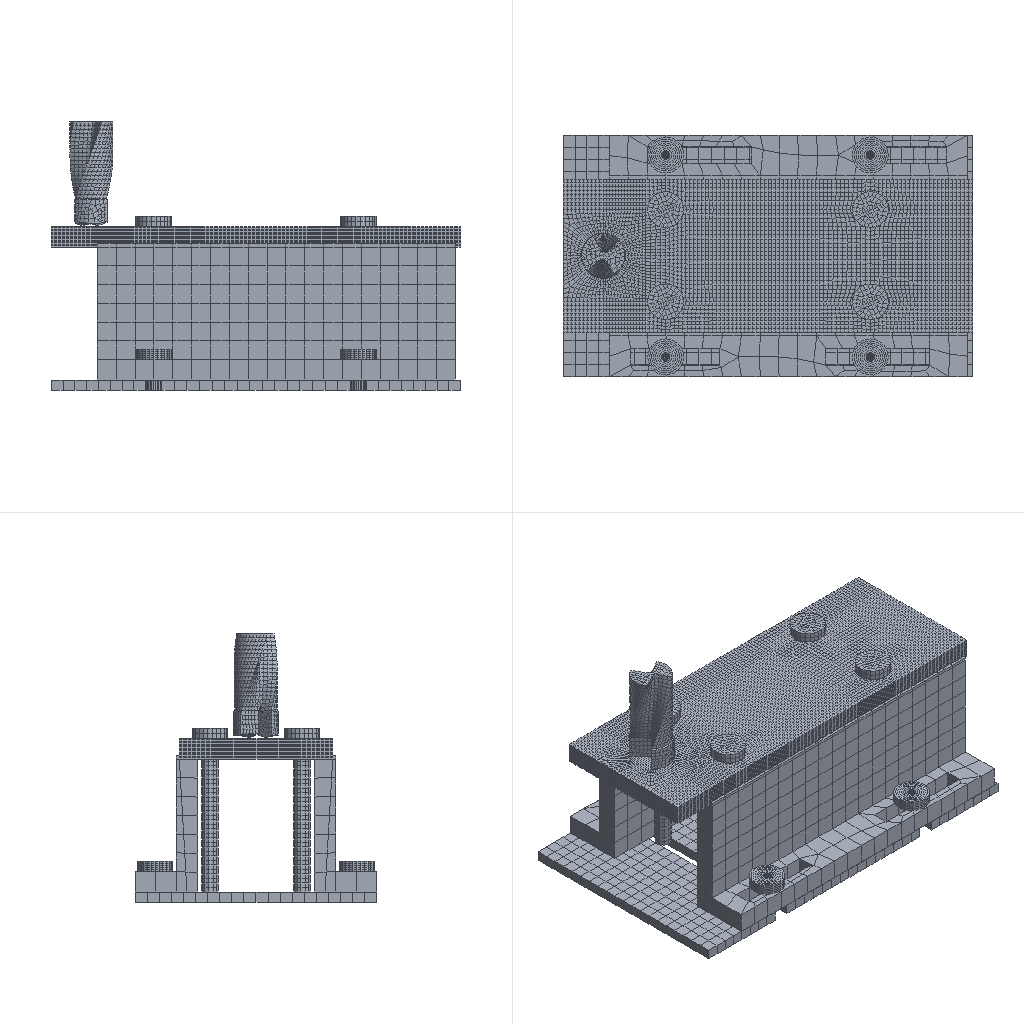Simulation study | abaqus
Set-up summary:
category,name,step,type,value,unit,region
solver,abaqus
solver,version,,,Abaqus/Standard 2024
units,not stated in the deck,,not stated
analysis,deck,,static,static
load_step,Step-1,Step-1,static,nlgeom=True
contact,interactions,,,general=0 pairs=22 ties=0
load_step,requested,,,1
mesh,nodes,,,96608
mesh,elements,,,84368
element_type,S3,,shell,42
element_type,S4R,,shell,1138
element_type,C3D8R,,solid,3884
element_type,C3D8RT,,solid,79304
load,load commands in deck,,count,4
bc,support commands in deck,,count,3
material,AL2219,,in results
material,AL2219-COPY,,in results
material,STEEL,,in results
check,setup vs results,,match,"per instance, exact: element labels, types and connectivity; labels of the nodes the elements use; coordinates of those nodes at SINGLE_PRECISION in 15 of 15 instance(s)"
Abaqus input file, long lists of numbers shortened, first 397 of 2407 lines:
*Heading
** Job name: yujing4 Model name: Model-1-Copy
** Generated by: Abaqus/CAE 2024
*Preprint, echo=NO, model=NO, history=NO, contact=NO
**
** PARTS
**
*Part, name=U44
*Node
      1,          76.,    14.767,  -16.307
      2,   97.892,    14.767,  -16.307
** (1159 more lines like these left out)
*Element, type=S4R
 1,   1,  57, 362,   4
 2,  57,  58, 363, 362
** (1136 more lines like these left out)
*Element, type=S3
873,   5,   6, 348
874, 344, 348,   6
** (40 more lines like these left out)
*Nset, nset=_PickedSet5, internal, generate
    1,  1161,     1
*Elset, elset=_PickedSet5, internal, generate
    1,  1180,     1
** Section: Section-4
*Shell Section, elset=_PickedSet5, material=steel
1., 5
*End Part
**
*Part, name=ban
*Node
      1,         150.,         -45.,           0.
      2,         150.,         -45.,          20.
** (71070 more lines like these left out)
*Element, type=C3D8RT
   1,  3164,  3165, 23216, 23000,   140,   139,  2928,  2927
   2,  3165,  3166, 23217, 23216,   139,   138,  2929,  2928
** (64018 more lines like these left out)
*Nset, nset=_PickedSet25, internal, generate
     1,  71072,      1
*Elset, elset=_PickedSet25, internal, generate
     1,  64020,      1
*Orientation, name=Ori-3
1., 0., 0., 0., 1., 0.
1, 0.
** Section: Section-2
*Solid Section, elset=_PickedSet25, orientation=Ori-3, material=AL2219
,
*End Part
**
*Part, name=diban1
*Node
      1,        -118.,          46.,           0.
      2,        -118.,         34.5,           0.
** (376 more lines like these left out)
*Element, type=C3D8R
  1,  19,  20,  29,  28,   1,   2,  11,  10
  2,  20,  21,  30,  29,   2,   3,  12,  11
** (158 more lines like these left out)
*Node
    379,           0.,           0.,          10.
*Nset, nset=diban1-RefPt_, internal
379,
*Nset, nset=_PickedSet2, internal, generate
   1,  378,    1
*Elset, elset=_PickedSet2, internal, generate
   1,  160,    1
** Section: steel
*Solid Section, elset=_PickedSet2, material=steel
,
*End Part
**
*Part, name=diban2
*Node
      1,        -118.,           0.,         -92.
      2,        -118.,           0.,  -79.733
** (670 more lines like these left out)
*Element, type=C3D8R
  1,  33,  34,  50,  49,   1,   2,  18,  17
  2,  34,  35,  51,  50,   2,   3,  19,  18
** (298 more lines like these left out)
*Node
    673,           0.,          10.,           0.
*Nset, nset=diban2-RefPt_, internal
673,
*Nset, nset=_PickedSet2, internal, generate
   1,  672,    1
*Elset, elset=_PickedSet2, internal, generate
   1,  300,    1
** Section: steel
*Solid Section, elset=_PickedSet2, material=steel
,
*End Part
**
*Part, name=dizuo
*Node
      1,   10.508,  -254.413,           0.
      2,   10.508,   95.587,           0.
** (650 more lines like these left out)
*Element, type=C3D8RT
  1,  11, 151, 545, 299,   1,  37, 281,  74
  2, 151, 152, 546, 545,  37,  38, 282, 281
** (336 more lines like these left out)
*Nset, nset=_PickedSet9, internal, generate
   1,  652,    1
*Elset, elset=_PickedSet9, internal, generate
   1,  338,    1
*Orientation, name=Ori-1
1., 0., 0., 0., 1., 0.
1, 0.
** Section: Section-3
*Solid Section, elset=_PickedSet9, orientation=Ori-1, material=AL2219-Copy
,
*End Part
**
*Part, name=luoshuan
*Node
      1,           0.,          -8.,          85.
      2,           0.,           0.,          85.
** (1159 more lines like these left out)
*Element, type=C3D8R
 1, 312, 313, 883, 874,  25,  26, 295, 294
 2, 313,  28, 296, 883,  26,   1,  27, 295
** (814 more lines like these left out)
*Nset, nset=_PickedSet2, internal, generate
    1,  1161,     1
*Elset, elset=_PickedSet2, internal, generate
   1,  816,    1
** Section: steel
*Solid Section, elset=_PickedSet2, material=steel
,
*End Part
**
*Part, name=luoshuan2
*Node
      1,           0.,          40.,  -4.142
      2,           0.,          40.,          -8.
** (4247 more lines like these left out)
*Element, type=C3D8RT
  1,  370,  397,   27,   28, 1840, 1867,  603,  604
  2,  374,   68,   69,  373, 1844,  452,  451, 1843
** (3650 more lines like these left out)
*Nset, nset=_PickedSet2, internal, generate
    1,  4249,     1
*Elset, elset=_PickedSet2, internal, generate
    1,  3652,     1
** Section: steel
*Solid Section, elset=_PickedSet2, material=steel
,
*End Part
**
**
** ASSEMBLY
**
*Assembly, name=Assembly
**
*Instance, name=diban2, part=diban2
-0.5575, 2.091,        -140.
-0.5575, 2.091,        -140., 0.01987, 2.668, -140.577,         240.
*End Instance
**
*Instance, name=luoshuan2, part=luoshuan2
99.443, -96.588,        -110.
99.443, -96.588,        -110., 98.443, -96.588,        -110., 90.
*End Instance
**
*Instance, name=luoshuan2_1, part=luoshuan2
99.443, 100.769,        -110.
99.443, 100.769,        -110., 98.443, 100.769,        -110., 90.
*End Instance
**
*Instance, name=diban1, part=diban1
153.443, 2.091,        -150.
153.443, 2.091,        -150., 153.443, 2.091, -149., 90.
*End Instance
**
*Instance, name=luoshuan2_2, part=luoshuan2
-100.557, 100.769,        -110.
-100.557, 100.769,        -110., -101.557, 100.769,        -110., 90.
*End Instance
**
*Instance, name=luoshuan2_3, part=luoshuan2
-100.557, -96.588,        -110.
-100.557, -96.588,        -110., -101.557, -96.588,        -110., 90.
*End Instance
**
*Instance, name=diban1_4, part=diban1
-154.557, 2.091,        -150.
-154.557, 2.091,        -150., -154.557, 2.091, -151., 90.
*End Instance
**
*Instance, name=dizuo, part=dizuo
-59.971, -86.418,        -140.
-59.971, -86.418,        -140., -59.971, -86.418, -139., 90.
*End Instance
**
*Instance, name=dizuo_5, part=dizuo
98.856, 90.599,        -140.
98.856, 90.599,        -140., 98.856, 90.599, -141., 90.
*End Instance
**
*Instance, name=luoshuan, part=luoshuan
99.443, 47.091,          20.
99.443, 47.091,          20., 99.247, 48.071,          20.,         180.
*End Instance
**
*Instance, name=luoshuan_6, part=luoshuan
99.443, -42.909,          20.
99.443, -42.909,          20., 99.247, -41.929,          20.,         180.
*End Instance
**
*Instance, name=luoshuan_7, part=luoshuan
-100.557, -42.909,          20.
-100.557, -42.909,          20., -100.753, -41.929,          20.,         180.
*End Instance
**
*Instance, name=luoshuan_8, part=luoshuan
-100.557, 47.091,          20.
-100.557, 47.091,          20., -100.753, 48.071,          20.,         180.
*End Instance
**
*Instance, name=ban, part=ban
-0.5575, 2.091,         -10.
*End Instance
**
*Instance, name=temp-U44钻头2025-2-new-1, part=U44
-161.557, 2.091, 112.448
-161.557, 2.091, 112.448, -161.557, 3.091, 112.448, 90.
*End Instance
**
*Nset, nset=Set-2, instance=ban
   107,   108,   109,   110,   119,   120,   122,   123,   129,   130,  2203,  2204,  2205,  2206,  2207,  2208
  2209,  2210,  2211,  2212,  2213,  2214,  2215,  2216,  2217,  2218,  2219,  2220,  2221,  2222,  2223,  2224
** (389 more lines like these left out)
*Nset, nset=_PickedSet283, internal, instance=luoshuan2
    1,    2,    7,    8,   15,   16,   21,   22,   26,   80,   81,   82,   83,   84,   85,   92
   93,   94,   95,   96,   97,  110,  170,  171,  172,  173,  174,  175,  176,  177,  178,  179
** (8 more lines like these left out)
*Nset, nset=_PickedSet283, internal, instance=luoshuan2_1
    1,    2,    7,    8,   15,   16,   21,   22,   26,   80,   81,   82,   83,   84,   85,   92
   93,   94,   95,   96,   97,  110,  170,  171,  172,  173,  174,  175,  176,  177,  178,  179
** (8 more lines like these left out)
*Nset, nset=_PickedSet283, internal, instance=luoshuan2_3
    1,    2,    7,    8,   15,   16,   21,   22,   26,   80,   81,   82,   83,   84,   85,   92
   93,   94,   95,   96,   97,  110,  170,  171,  172,  173,  174,  175,  176,  177,  178,  179
** (8 more lines like these left out)
*Nset, nset=_PickedSet283, internal, instance=luoshuan2_2
    1,    2,    7,    8,   15,   16,   21,   22,   26,   80,   81,   82,   83,   84,   85,   92
   93,   94,   95,   96,   97,  110,  170,  171,  172,  173,  174,  175,  176,  177,  178,  179
** (8 more lines like these left out)
*Elset, elset=_PickedSet283, internal, instance=luoshuan2
    5,   32,   74,  101,  143,  170,  212,  239,  281,  308,  350,  377,  419,  446,  488,  515
  557,  584,  626,  653,  695,  722,  764,  791,  833,  860,  902,  929,  971,  998, 1040, 1067
** (7 more lines like these left out)
*Elset, elset=_PickedSet283, internal, instance=luoshuan2_1
    5,   32,   74,  101,  143,  170,  212,  239,  281,  308,  350,  377,  419,  446,  488,  515
  557,  584,  626,  653,  695,  722,  764,  791,  833,  860,  902,  929,  971,  998, 1040, 1067
** (7 more lines like these left out)
*Elset, elset=_PickedSet283, internal, instance=luoshuan2_3
    5,   32,   74,  101,  143,  170,  212,  239,  281,  308,  350,  377,  419,  446,  488,  515
  557,  584,  626,  653,  695,  722,  764,  791,  833,  860,  902,  929,  971,  998, 1040, 1067
** (7 more lines like these left out)
*Elset, elset=_PickedSet283, internal, instance=luoshuan2_2
    5,   32,   74,  101,  143,  170,  212,  239,  281,  308,  350,  377,  419,  446,  488,  515
  557,  584,  626,  653,  695,  722,  764,  791,  833,  860,  902,  929,  971,  998, 1040, 1067
** (7 more lines like these left out)
*Nset, nset=_PickedSet284, internal, instance=luoshuan
   4,   5,   6,   8,  10,  78,  79,  80,  81,  82, 103, 104, 105, 106, 126, 127
 128, 223, 224, 376, 377, 444, 445, 496, 497, 730, 731
*Nset, nset=_PickedSet284, internal, instance=luoshuan_6
   4,   5,   6,   8,  10,  78,  79,  80,  81,  82, 103, 104, 105, 106, 126, 127
 128, 223, 224, 376, 377, 444, 445, 496, 497, 730, 731
*Nset, nset=_PickedSet284, internal, instance=luoshuan_7
   4,   5,   6,   8,  10,  78,  79,  80,  81,  82, 103, 104, 105, 106, 126, 127
 128, 223, 224, 376, 377, 444, 445, 496, 497, 730, 731
*Nset, nset=_PickedSet284, internal, instance=luoshuan_8
   4,   5,   6,   8,  10,  78,  79,  80,  81,  82, 103, 104, 105, 106, 126, 127
 128, 223, 224, 376, 377, 444, 445, 496, 497, 730, 731
*Elset, elset=_PickedSet284, internal, instance=luoshuan
  49,  58,  59,  68,  85, 134, 135, 136, 161, 170, 219, 220, 221, 246, 255, 545
 553, 554, 580, 581
*Elset, elset=_PickedSet284, internal, instance=luoshuan_6
  49,  58,  59,  68,  85, 134, 135, 136, 161, 170, 219, 220, 221, 246, 255, 545
 553, 554, 580, 581
*Elset, elset=_PickedSet284, internal, instance=luoshuan_7
  49,  58,  59,  68,  85, 134, 135, 136, 161, 170, 219, 220, 221, 246, 255, 545
 553, 554, 580, 581
*Elset, elset=_PickedSet284, internal, instance=luoshuan_8
  49,  58,  59,  68,  85, 134, 135, 136, 161, 170, 219, 220, 221, 246, 255, 545
 553, 554, 580, 581
*Nset, nset=_PickedSet291, internal, instance=diban2
 673,
*Nset, nset=_PickedSet291, internal, instance=diban1
 379,
*Nset, nset=_PickedSet291, internal, instance=diban1_4
 379,
*Nset, nset=_PickedSet292, internal, instance=diban1_4
 379,
*Nset, nset=_PickedSet293, internal, instance=diban1_4, generate
   1,  378,    1
*Elset, elset=_PickedSet293, internal, instance=diban1_4, generate
   1,  160,    1
*Nset, nset=_PickedSet294, internal, instance=diban2
 673,
*Nset, nset=_PickedSet295, internal, instance=diban2, generate
   1,  672,    1
*Elset, elset=_PickedSet295, internal, instance=diban2, generate
   1,  300,    1
*Nset, nset=_PickedSet296, internal, instance=diban1
 379,
*Nset, nset=_PickedSet297, internal, instance=diban1, generate
   1,  378,    1
*Elset, elset=_PickedSet297, internal, instance=diban1, generate
   1,  160,    1
*Elset, elset=_CP-1-diban2_S3, internal, instance=diban2, generate
   1,  300,    1
*Surface, type=ELEMENT, name=CP-1-diban2
_CP-1-diban2_S3, S3
*Elset, elset=_CP-1-dizuo_S1, internal, instance=dizuo, generate
 286,  338,    1
*Elset, elset=_CP-1-dizuo_S2, internal, instance=dizuo, generate
  1,  38,   1
*Surface, type=ELEMENT, name=CP-1-dizuo
_CP-1-dizuo_S1, S1
_CP-1-dizuo_S2, S2
*Elset, elset=_CP-2-diban2_S3, internal, instance=diban2, generate
   1,  300,    1
*Surface, type=ELEMENT, name=CP-2-diban2
_CP-2-diban2_S3, S3
*Elset, elset=_CP-2-dizuo_S1, internal, instance=dizuo, generate
 286,  338,    1
*Elset, elset=_CP-2-dizuo_S2, internal, instance=dizuo, generate
  1,  38,   1
*Surface, type=ELEMENT, name=CP-2-dizuo
_CP-2-dizuo_S1, S1
_CP-2-dizuo_S2, S2
*Elset, elset=_CP-2-dizuo_5_S1, internal, instance=dizuo_5, generate
 286,  338,    1
*Elset, elset=_CP-2-dizuo_5_S2, internal, instance=dizuo_5, generate
  1,  38,   1
*Surface, type=ELEMENT, name=CP-2-dizuo_5
_CP-2-dizuo_5_S1, S1
_CP-2-dizuo_5_S2, S2
*Elset, elset=_CP-3-diban2_S3, internal, instance=diban2, generate
   1,  300,    1
*Surface, type=ELEMENT, name=CP-3-diban2
_CP-3-diban2_S3, S3
*Elset, elset=_CP-3-dizuo_S2, internal, instance=dizuo, generate
 286,  338,    1
*Surface, type=ELEMENT, name=CP-3-dizuo
_CP-3-dizuo_S2, S2
*Elset, elset=_CP-3-dizuo_5_S1, internal, instance=dizuo_5, generate
 286,  338,    1
*Elset, elset=_CP-3-dizuo_5_S2, internal, instance=dizuo_5, generate
  1,  38,   1
*Surface, type=ELEMENT, name=CP-3-dizuo_5
_CP-3-dizuo_5_S1, S1
_CP-3-dizuo_5_S2, S2
*Elset, elset=_CP-3-luoshuan2_S3, internal, instance=luoshuan2
   19,   21,   49,   51,   88,   90,  118,  120,  157,  159,  187,  189,  226,  228,  256,  258
  295,  297,  325,  327,  364,  366,  394,  396,  433,  435,  463,  465,  502,  504,  532,  534
** (5 more lines like these left out)
*Elset, elset=_CP-3-luoshuan2_S5, internal, instance=luoshuan2, generate
   22,  1885,    69
*Surface, type=ELEMENT, name=CP-3-luoshuan2
_CP-3-luoshuan2_S3, S3
_CP-3-luoshuan2_S5, S5
*Elset, elset=_CP-4-diban2_S3, internal, instance=diban2, generate
   1,  300,    1
*Surface, type=ELEMENT, name=CP-4-diban2
_CP-4-diban2_S3, S3
*Elset, elset=_CP-4-dizuo_S4, internal, instance=dizuo
 292, 306
*Elset, elset=_CP-4-dizuo_S6, internal, instance=dizuo
 305, 307, 315, 316
*Surface, type=ELEMENT, name=CP-4-dizuo
_CP-4-dizuo_S4, S4
_CP-4-dizuo_S6, S6
*Elset, elset=_CP-4-dizuo_5_S1, internal, instance=dizuo_5, generate
 286,  338,    1
*Elset, elset=_CP-4-dizuo_5_S2, internal, instance=dizuo_5, generate
  1,  38,   1
*Surface, type=ELEMENT, name=CP-4-dizuo_5
_CP-4-dizuo_5_S1, S1
_CP-4-dizuo_5_S2, S2
*Elset, elset=_CP-4-luoshuan2_S5, internal, instance=luoshuan2
    1,    7,    8,    9,   10,   11,   12,   13,   14,   15,   16,   17,   18,   59,   70,   76
   77,   78,   79,   80,   81,   82,   83,   84,   85,   86,   87,  128,  139,  145,  146,  147
** (23 more lines like these left out)
*Elset, elset=_CP-4-luoshuan2_S3, internal, instance=luoshuan2, generate
    5,  1868,    69
*Surface, type=ELEMENT, name=CP-4-luoshuan2
_CP-4-luoshuan2_S5, S5
_CP-4-luoshuan2_S3, S3
*Elset, elset=_CP-5-diban2_S3, internal, instance=diban2, generate
   1,  300,    1
*Surface, type=ELEMENT, name=CP-5-diban2
Last 646 lines:
   366,   372,   378,   384,   390,   396,   402,   408,   414,   420,   426,   432,   438,   444,   450,   456
   462,   468,   474,   480,   486,   492,   498,   504,   510,   516,   522,   528,   534,   540,   546,   552
** (18 more lines like these left out)
*Elset, elset=_CP-40-ban_S2, internal, instance=ban
 22126, 22127, 22128, 22129, 22130, 22131, 22132, 22133, 22134, 22135, 22136, 22137, 22138, 22139, 22140, 22141
 22222, 22223, 22224, 22225, 22226, 22227, 22228, 22229, 22230, 22231, 22232, 22233, 22234, 22235, 39413, 39414
** (11 more lines like these left out)
*Elset, elset=_CP-40-ban_S6, internal, instance=ban, generate
 35866,  37418,      8
*Surface, type=ELEMENT, name=CP-40-ban
_CP-40-ban_S5, S5
_CP-40-ban_S3, S3
_CP-40-ban_S4, S4
_CP-40-ban_S2, S2
_CP-40-ban_S6, S6
*Elset, elset=_CP-40-dizuo_S2, internal, instance=dizuo, generate
 286,  338,    1
*Surface, type=ELEMENT, name=CP-40-dizuo
_CP-40-dizuo_S2, S2
*Elset, elset=_CP-40-dizuo_5_S4, internal, instance=dizuo_5
 292, 306
*Elset, elset=_CP-40-dizuo_5_S6, internal, instance=dizuo_5
 305, 307, 315, 316
*Surface, type=ELEMENT, name=CP-40-dizuo_5
_CP-40-dizuo_5_S4, S4
_CP-40-dizuo_5_S6, S6
*Elset, elset=_CP-41-ban_S6, internal, instance=ban
  5551,  5566,  5581,  5596,  5611,  5626,  5641,  5656,  5671,  5686,  5701,  5716,  5731,  5746,  5761,  5776
  5791,  5806,  5821,  5836,  5851,  5866,  5881,  5896,  5911,  5926,  5941,  5956,  5971,  5986,  6001,  6016
** (66 more lines like these left out)
*Elset, elset=_CP-41-ban_S5, internal, instance=ban
  9410,  9411,  9412,  9413,  9414,  9415,  9416,  9417,  9418,  9419,  9420,  9575,  9576,  9577,  9578,  9579
  9580,  9581,  9582,  9583,  9584,  9585,  9740,  9741,  9742,  9743,  9744,  9745,  9746,  9747,  9748,  9749
** (7 more lines like these left out)
*Elset, elset=_CP-41-ban_S4, internal, instance=ban
     8,    16,    24,    32,    40,    48,    56,    64,    72,    80,    88,    96,   104,   112,   120,   128
   136,   144,   152,   160,   168,   176,   830,   838,   846,   854,   862,   870,   878,   886,   894,   902
** (104 more lines like these left out)
*Elset, elset=_CP-41-ban_S3, internal, instance=ban
   345,   353,  1449,  1450,  1465,  1466,  1467,  1468,  1469,  1470,  1513,  1514,  1515,  1516,  1517,  1518
  2881,  2882,  2883,  2902,  2903,  2904,  2923,  2924,  2925,  2944,  2945,  2946,  2965,  2966,  2967,  2986
** (55 more lines like these left out)
*Elset, elset=_CP-41-ban_S2, internal, instance=ban
  3549, 12586, 12587, 12602, 12603, 12604, 12605, 12606, 12607, 12608, 12609, 12610, 12611, 18916, 18917, 18918
 18919, 18920, 18921, 18922, 18923, 18924, 18925, 18996, 18997, 20791, 20792, 20793, 20794, 20795, 20796, 20797
** (27 more lines like these left out)
*Surface, type=ELEMENT, name=CP-41-ban
_CP-41-ban_S6, S6
_CP-41-ban_S5, S5
_CP-41-ban_S4, S4
_CP-41-ban_S2, S2
_CP-41-ban_S3, S3
*Elset, elset=_CP-41-dizuo_S1, internal, instance=dizuo, generate
 286,  338,    1
*Elset, elset=_CP-41-dizuo_S2, internal, instance=dizuo, generate
  1,  38,   1
*Surface, type=ELEMENT, name=CP-41-dizuo
_CP-41-dizuo_S1, S1
_CP-41-dizuo_S2, S2
*Elset, elset=_CP-41-dizuo_5_S2, internal, instance=dizuo_5, generate
 286,  338,    1
*Surface, type=ELEMENT, name=CP-41-dizuo_5
_CP-41-dizuo_5_S2, S2
*Elset, elset=_CP-42-ban_S4, internal, instance=ban
 11735, 11740, 11745, 11750, 11755, 11760, 11765, 11770, 11775, 11780, 11785, 11790, 11795, 11800, 11805, 11810
 11815, 11820, 11825, 11830, 11835, 11840, 11845, 11850, 11855, 11860, 11865, 11870, 11875, 11880, 11885, 11890
** (21 more lines like these left out)
*Elset, elset=_CP-42-ban_S3, internal, instance=ban
 12171, 12172, 12173, 12174, 12175, 12176, 12177, 12206, 12207, 12208, 12209, 12210, 12211, 12212, 12241, 12242
 12243, 12244, 12245, 12246, 12247, 12276, 12277, 12278, 12279, 12280, 12281, 12282, 12311, 12312, 12313, 12314
** (16 more lines like these left out)
*Elset, elset=_CP-42-ban_S5, internal, instance=ban
 12856, 12857, 12858, 12859, 12860, 12861, 12862, 12863, 12864, 12865, 12866, 12867, 12868, 12869, 12870, 12961
 12962, 12963, 12964, 12965, 12966, 12967, 12968, 12969, 12970, 12971, 12972, 12973, 12974, 12975, 13066, 13067
** (36 more lines like these left out)
*Elset, elset=_CP-42-ban_S2, internal, instance=ban
 19012, 19013, 19014, 19015, 19016, 19017, 19018, 19019, 19020, 19021, 19022, 19023, 19024, 19025, 46141, 46142
 46143, 46144, 46145, 46146, 46147, 46148, 46149, 46150, 46151, 46152, 46153, 46154, 46155, 46156, 46157, 46158
** (21 more lines like these left out)
*Surface, type=ELEMENT, name=CP-42-ban
_CP-42-ban_S4, S4
_CP-42-ban_S3, S3
_CP-42-ban_S2, S2
_CP-42-ban_S5, S5
*Elset, elset=_CP-42-dizuo_S1, internal, instance=dizuo, generate
 248,  266,    1
*Surface, type=ELEMENT, name=CP-42-dizuo
_CP-42-dizuo_S1, S1
*Elset, elset=_CP-42-dizuo_5_S1, internal, instance=dizuo_5, generate
 286,  338,    1
*Elset, elset=_CP-42-dizuo_5_S2, internal, instance=dizuo_5, generate
  1,  38,   1
*Surface, type=ELEMENT, name=CP-42-dizuo_5
_CP-42-dizuo_5_S1, S1
_CP-42-dizuo_5_S2, S2
*Elset, elset=_CP-43-ban_S3, internal, instance=ban
   177,   178,   179,   180,   181,   182,   183,   184,   185,   186,   187,   254,   255,   256,   257,   258
   259,   260,   261,   262,   263,   264,   361,   362,   363,   364,   365,   366,   403,   404,   405,   406
** (88 more lines like these left out)
*Elset, elset=_CP-43-ban_S4, internal, instance=ban
   337,   344,  3119,  3127,  3135,  3143,  3151,  3159,  3167,  3175,  3183,  3191,  3199,  3207,  3215,  3223
  3231,  3239,  3247,  3255,  3263,  3271,  3279,  3287,  3295,  3303,  3311,  3319,  3327,  3335,  3343,  3351
** (116 more lines like these left out)
*Elset, elset=_CP-43-ban_S2, internal, instance=ban
  1351,  1352,  1365,  1366,  1367,  1368,  1369,  1370,  1371,  1372,  1373,  1374,  1375,  1376,  3496,  3497
  3498,  3520,  5371,  5372,  5373,  5374,  5375,  5376,  5377,  5378,  5427,  5434,  5435,  5436, 19082, 19083
** (20 more lines like these left out)
*Elset, elset=_CP-43-ban_S6, internal, instance=ban
  7111,  7126,  7141,  7156,  7171,  7186,  7201,  7216,  7231,  7246,  7261,  7276,  7291,  7306,  7321,  7336
  7351,  7366,  7381,  7396,  7411,  7426,  7441,  7456,  7471,  7486,  7501,  7516,  7531,  7546,  7561,  7576
** (30 more lines like these left out)
*Elset, elset=_CP-43-ban_S1, internal, instance=ban, generate
 37322,  37425,      1
*Surface, type=ELEMENT, name=CP-43-ban
_CP-43-ban_S3, S3
_CP-43-ban_S4, S4
_CP-43-ban_S2, S2
_CP-43-ban_S6, S6
_CP-43-ban_S1, S1
*Elset, elset=_CP-43-dizuo_S6, internal, instance=dizuo, generate
 267,  285,    1
*Surface, type=ELEMENT, name=CP-43-dizuo
_CP-43-dizuo_S6, S6
*Elset, elset=_CP-43-dizuo_5_S1, internal, instance=dizuo_5, generate
 248,  266,    1
*Surface, type=ELEMENT, name=CP-43-dizuo_5
_CP-43-dizuo_5_S1, S1
*Elset, elset=_CP-44-ban_S3, internal, instance=ban
   177,   178,   179,   180,   181,   182,   183,   184,   185,   186,   187,   254,   255,   256,   257,   258
   259,   260,   261,   262,   263,   264,   361,   362,   363,   364,   365,   366,   403,   404,   405,   406
** (88 more lines like these left out)
*Elset, elset=_CP-44-ban_S4, internal, instance=ban
   337,   344,  3119,  3127,  3135,  3143,  3151,  3159,  3167,  3175,  3183,  3191,  3199,  3207,  3215,  3223
  3231,  3239,  3247,  3255,  3263,  3271,  3279,  3287,  3295,  3303,  3311,  3319,  3327,  3335,  3343,  3351
** (116 more lines like these left out)
*Elset, elset=_CP-44-ban_S2, internal, instance=ban
  1351,  1352,  1365,  1366,  1367,  1368,  1369,  1370,  1371,  1372,  1373,  1374,  1375,  1376,  3496,  3497
  3498,  3520,  5371,  5372,  5373,  5374,  5375,  5376,  5377,  5378,  5427,  5434,  5435,  5436, 19082, 19083
** (20 more lines like these left out)
*Elset, elset=_CP-44-ban_S6, internal, instance=ban
  7111,  7126,  7141,  7156,  7171,  7186,  7201,  7216,  7231,  7246,  7261,  7276,  7291,  7306,  7321,  7336
  7351,  7366,  7381,  7396,  7411,  7426,  7441,  7456,  7471,  7486,  7501,  7516,  7531,  7546,  7561,  7576
** (30 more lines like these left out)
*Elset, elset=_CP-44-ban_S1, internal, instance=ban, generate
 37322,  37425,      1
*Surface, type=ELEMENT, name=CP-44-ban
_CP-44-ban_S3, S3
_CP-44-ban_S4, S4
_CP-44-ban_S2, S2
_CP-44-ban_S6, S6
_CP-44-ban_S1, S1
*Elset, elset=_CP-44-dizuo_5_S6, internal, instance=dizuo_5, generate
 267,  285,    1
*Surface, type=ELEMENT, name=CP-44-dizuo_5
_CP-44-dizuo_5_S6, S6
*Elset, elset=_CP-45-ban_S3, internal, instance=ban
   177,   178,   179,   180,   181,   182,   183,   184,   185,   186,   187,   254,   255,   256,   257,   258
   259,   260,   261,   262,   263,   264,   361,   362,   363,   364,   365,   366,   403,   404,   405,   406
** (88 more lines like these left out)
*Elset, elset=_CP-45-ban_S4, internal, instance=ban
   337,   344,  3119,  3127,  3135,  3143,  3151,  3159,  3167,  3175,  3183,  3191,  3199,  3207,  3215,  3223
  3231,  3239,  3247,  3255,  3263,  3271,  3279,  3287,  3295,  3303,  3311,  3319,  3327,  3335,  3343,  3351
** (116 more lines like these left out)
*Elset, elset=_CP-45-ban_S2, internal, instance=ban
  1351,  1352,  1365,  1366,  1367,  1368,  1369,  1370,  1371,  1372,  1373,  1374,  1375,  1376,  3496,  3497
  3498,  3520,  5371,  5372,  5373,  5374,  5375,  5376,  5377,  5378,  5427,  5434,  5435,  5436, 19082, 19083
** (20 more lines like these left out)
*Elset, elset=_CP-45-ban_S6, internal, instance=ban
  7111,  7126,  7141,  7156,  7171,  7186,  7201,  7216,  7231,  7246,  7261,  7276,  7291,  7306,  7321,  7336
  7351,  7366,  7381,  7396,  7411,  7426,  7441,  7456,  7471,  7486,  7501,  7516,  7531,  7546,  7561,  7576
** (30 more lines like these left out)
*Elset, elset=_CP-45-ban_S1, internal, instance=ban, generate
 37322,  37425,      1
*Surface, type=ELEMENT, name=CP-45-ban
_CP-45-ban_S3, S3
_CP-45-ban_S4, S4
_CP-45-ban_S2, S2
_CP-45-ban_S6, S6
_CP-45-ban_S1, S1
*Elset, elset=_CP-46-ban_S3, internal, instance=ban
   177,   178,   179,   180,   181,   182,   183,   184,   185,   186,   187,   254,   255,   256,   257,   258
   259,   260,   261,   262,   263,   264,   361,   362,   363,   364,   365,   366,   403,   404,   405,   406
** (88 more lines like these left out)
*Elset, elset=_CP-46-ban_S4, internal, instance=ban
   337,   344,  3119,  3127,  3135,  3143,  3151,  3159,  3167,  3175,  3183,  3191,  3199,  3207,  3215,  3223
  3231,  3239,  3247,  3255,  3263,  3271,  3279,  3287,  3295,  3303,  3311,  3319,  3327,  3335,  3343,  3351
** (116 more lines like these left out)
*Elset, elset=_CP-46-ban_S2, internal, instance=ban
  1351,  1352,  1365,  1366,  1367,  1368,  1369,  1370,  1371,  1372,  1373,  1374,  1375,  1376,  3496,  3497
  3498,  3520,  5371,  5372,  5373,  5374,  5375,  5376,  5377,  5378,  5427,  5434,  5435,  5436, 19082, 19083
** (20 more lines like these left out)
*Elset, elset=_CP-46-ban_S6, internal, instance=ban
  7111,  7126,  7141,  7156,  7171,  7186,  7201,  7216,  7231,  7246,  7261,  7276,  7291,  7306,  7321,  7336
  7351,  7366,  7381,  7396,  7411,  7426,  7441,  7456,  7471,  7486,  7501,  7516,  7531,  7546,  7561,  7576
** (30 more lines like these left out)
*Elset, elset=_CP-46-ban_S1, internal, instance=ban, generate
 37322,  37425,      1
*Surface, type=ELEMENT, name=CP-46-ban
_CP-46-ban_S3, S3
_CP-46-ban_S4, S4
_CP-46-ban_S2, S2
_CP-46-ban_S6, S6
_CP-46-ban_S1, S1
*Elset, elset=_CP-47-ban_S6, internal, instance=ban
  5551,  5566,  5581,  5596,  5611,  5626,  5641,  5656,  5671,  5686,  5701,  5716,  5731,  5746,  5761,  5776
  5791,  5806,  5821,  5836,  5851,  5866,  5881,  5896,  5911,  5926,  5941,  5956,  5971,  5986,  6001,  6016
** (66 more lines like these left out)
*Elset, elset=_CP-47-ban_S5, internal, instance=ban
  9410,  9411,  9412,  9413,  9414,  9415,  9416,  9417,  9418,  9419,  9420,  9575,  9576,  9577,  9578,  9579
  9580,  9581,  9582,  9583,  9584,  9585,  9740,  9741,  9742,  9743,  9744,  9745,  9746,  9747,  9748,  9749
** (7 more lines like these left out)
*Elset, elset=_CP-47-ban_S4, internal, instance=ban
     8,    16,    24,    32,    40,    48,    56,    64,    72,    80,    88,    96,   104,   112,   120,   128
   136,   144,   152,   160,   168,   176,   830,   838,   846,   854,   862,   870,   878,   886,   894,   902
** (104 more lines like these left out)
*Elset, elset=_CP-47-ban_S3, internal, instance=ban
   345,   353,  1449,  1450,  1465,  1466,  1467,  1468,  1469,  1470,  1513,  1514,  1515,  1516,  1517,  1518
  2881,  2882,  2883,  2902,  2903,  2904,  2923,  2924,  2925,  2944,  2945,  2946,  2965,  2966,  2967,  2986
** (55 more lines like these left out)
*Elset, elset=_CP-47-ban_S2, internal, instance=ban
  3549, 12586, 12587, 12602, 12603, 12604, 12605, 12606, 12607, 12608, 12609, 12610, 12611, 18916, 18917, 18918
 18919, 18920, 18921, 18922, 18923, 18924, 18925, 18996, 18997, 20791, 20792, 20793, 20794, 20795, 20796, 20797
** (27 more lines like these left out)
*Surface, type=ELEMENT, name=CP-47-ban
_CP-47-ban_S6, S6
_CP-47-ban_S5, S5
_CP-47-ban_S4, S4
_CP-47-ban_S2, S2
_CP-47-ban_S3, S3
*Elset, elset=_CP-48-ban_S5, internal, instance=ban
  5656,  5657,  5658,  5659,  5660,  5661,  5662,  5663,  5664,  5665,  5666,  5667,  5668,  5669,  5670,  5776
  5777,  5778,  5779,  5780,  5781,  5782,  5783,  5784,  5785,  5786,  5787,  5788,  5789,  5790,  5896,  5897
** (36 more lines like these left out)
*Elset, elset=_CP-48-ban_S3, internal, instance=ban
   823,   824,   825,   826,   827,   828,   829,   830,   871,   872,   873,   874,   875,   876,   877,   878
   919,   920,   921,   922,   923,   924,   925,   926,   967,   968,   969,   970,   971,   972,   973,   974
** (16 more lines like these left out)
*Elset, elset=_CP-48-ban_S4, internal, instance=ban
   366,   372,   378,   384,   390,   396,   402,   408,   414,   420,   426,   432,   438,   444,   450,   456
   462,   468,   474,   480,   486,   492,   498,   504,   510,   516,   522,   528,   534,   540,   546,   552
** (18 more lines like these left out)
*Elset, elset=_CP-48-ban_S2, internal, instance=ban
 22126, 22127, 22128, 22129, 22130, 22131, 22132, 22133, 22134, 22135, 22136, 22137, 22138, 22139, 22140, 22141
 22222, 22223, 22224, 22225, 22226, 22227, 22228, 22229, 22230, 22231, 22232, 22233, 22234, 22235, 39413, 39414
** (11 more lines like these left out)
*Elset, elset=_CP-48-ban_S6, internal, instance=ban, generate
 35866,  37418,      8
*Surface, type=ELEMENT, name=CP-48-ban
_CP-48-ban_S5, S5
_CP-48-ban_S3, S3
_CP-48-ban_S4, S4
_CP-48-ban_S2, S2
_CP-48-ban_S6, S6
*Elset, elset=_CP-49-ban_S6, internal, instance=ban
  5551,  5566,  5581,  5596,  5611,  5626,  5641,  5656,  5671,  5686,  5701,  5716,  5731,  5746,  5761,  5776
  5791,  5806,  5821,  5836,  5851,  5866,  5881,  5896,  5911,  5926,  5941,  5956,  5971,  5986,  6001,  6016
** (66 more lines like these left out)
*Elset, elset=_CP-49-ban_S5, internal, instance=ban
  9410,  9411,  9412,  9413,  9414,  9415,  9416,  9417,  9418,  9419,  9420,  9575,  9576,  9577,  9578,  9579
  9580,  9581,  9582,  9583,  9584,  9585,  9740,  9741,  9742,  9743,  9744,  9745,  9746,  9747,  9748,  9749
** (7 more lines like these left out)
*Elset, elset=_CP-49-ban_S4, internal, instance=ban
     8,    16,    24,    32,    40,    48,    56,    64,    72,    80,    88,    96,   104,   112,   120,   128
   136,   144,   152,   160,   168,   176,   830,   838,   846,   854,   862,   870,   878,   886,   894,   902
** (104 more lines like these left out)
*Elset, elset=_CP-49-ban_S3, internal, instance=ban
   345,   353,  1449,  1450,  1465,  1466,  1467,  1468,  1469,  1470,  1513,  1514,  1515,  1516,  1517,  1518
  2881,  2882,  2883,  2902,  2903,  2904,  2923,  2924,  2925,  2944,  2945,  2946,  2965,  2966,  2967,  2986
** (55 more lines like these left out)
*Elset, elset=_CP-49-ban_S2, internal, instance=ban
  3549, 12586, 12587, 12602, 12603, 12604, 12605, 12606, 12607, 12608, 12609, 12610, 12611, 18916, 18917, 18918
 18919, 18920, 18921, 18922, 18923, 18924, 18925, 18996, 18997, 20791, 20792, 20793, 20794, 20795, 20796, 20797
** (27 more lines like these left out)
*Surface, type=ELEMENT, name=CP-49-ban
_CP-49-ban_S6, S6
_CP-49-ban_S5, S5
_CP-49-ban_S4, S4
_CP-49-ban_S2, S2
_CP-49-ban_S3, S3
*Elset, elset=_CP-50-ban_S4, internal, instance=ban
 11735, 11740, 11745, 11750, 11755, 11760, 11765, 11770, 11775, 11780, 11785, 11790, 11795, 11800, 11805, 11810
 11815, 11820, 11825, 11830, 11835, 11840, 11845, 11850, 11855, 11860, 11865, 11870, 11875, 11880, 11885, 11890
** (21 more lines like these left out)
*Elset, elset=_CP-50-ban_S3, internal, instance=ban
 12171, 12172, 12173, 12174, 12175, 12176, 12177, 12206, 12207, 12208, 12209, 12210, 12211, 12212, 12241, 12242
 12243, 12244, 12245, 12246, 12247, 12276, 12277, 12278, 12279, 12280, 12281, 12282, 12311, 12312, 12313, 12314
** (16 more lines like these left out)
*Elset, elset=_CP-50-ban_S5, internal, instance=ban
 12856, 12857, 12858, 12859, 12860, 12861, 12862, 12863, 12864, 12865, 12866, 12867, 12868, 12869, 12870, 12961
 12962, 12963, 12964, 12965, 12966, 12967, 12968, 12969, 12970, 12971, 12972, 12973, 12974, 12975, 13066, 13067
** (36 more lines like these left out)
*Elset, elset=_CP-50-ban_S2, internal, instance=ban
 19012, 19013, 19014, 19015, 19016, 19017, 19018, 19019, 19020, 19021, 19022, 19023, 19024, 19025, 46141, 46142
 46143, 46144, 46145, 46146, 46147, 46148, 46149, 46150, 46151, 46152, 46153, 46154, 46155, 46156, 46157, 46158
** (21 more lines like these left out)
*Surface, type=ELEMENT, name=CP-50-ban
_CP-50-ban_S4, S4
_CP-50-ban_S3, S3
_CP-50-ban_S2, S2
_CP-50-ban_S5, S5
*Elset, elset=_CP-51-ban_S3, internal, instance=ban
   177,   178,   179,   180,   181,   182,   183,   184,   185,   186,   187,   254,   255,   256,   257,   258
   259,   260,   261,   262,   263,   264,   361,   362,   363,   364,   365,   366,   403,   404,   405,   406
** (88 more lines like these left out)
*Elset, elset=_CP-51-ban_S4, internal, instance=ban
   337,   344,  3119,  3127,  3135,  3143,  3151,  3159,  3167,  3175,  3183,  3191,  3199,  3207,  3215,  3223
  3231,  3239,  3247,  3255,  3263,  3271,  3279,  3287,  3295,  3303,  3311,  3319,  3327,  3335,  3343,  3351
** (116 more lines like these left out)
*Elset, elset=_CP-51-ban_S2, internal, instance=ban
  1351,  1352,  1365,  1366,  1367,  1368,  1369,  1370,  1371,  1372,  1373,  1374,  1375,  1376,  3496,  3497
  3498,  3520,  5371,  5372,  5373,  5374,  5375,  5376,  5377,  5378,  5427,  5434,  5435,  5436, 19082, 19083
** (20 more lines like these left out)
*Elset, elset=_CP-51-ban_S6, internal, instance=ban
  7111,  7126,  7141,  7156,  7171,  7186,  7201,  7216,  7231,  7246,  7261,  7276,  7291,  7306,  7321,  7336
  7351,  7366,  7381,  7396,  7411,  7426,  7441,  7456,  7471,  7486,  7501,  7516,  7531,  7546,  7561,  7576
** (30 more lines like these left out)
*Elset, elset=_CP-51-ban_S1, internal, instance=ban, generate
 37322,  37425,      1
*Surface, type=ELEMENT, name=CP-51-ban
_CP-51-ban_S3, S3
_CP-51-ban_S4, S4
_CP-51-ban_S2, S2
_CP-51-ban_S6, S6
_CP-51-ban_S1, S1
*Elset, elset=_CP-52-ban_S3, internal, instance=ban
   177,   178,   179,   180,   181,   182,   183,   184,   185,   186,   187,   254,   255,   256,   257,   258
   259,   260,   261,   262,   263,   264,   361,   362,   363,   364,   365,   366,   403,   404,   405,   406
** (88 more lines like these left out)
*Elset, elset=_CP-52-ban_S4, internal, instance=ban
   337,   344,  3119,  3127,  3135,  3143,  3151,  3159,  3167,  3175,  3183,  3191,  3199,  3207,  3215,  3223
  3231,  3239,  3247,  3255,  3263,  3271,  3279,  3287,  3295,  3303,  3311,  3319,  3327,  3335,  3343,  3351
** (116 more lines like these left out)
*Elset, elset=_CP-52-ban_S2, internal, instance=ban
  1351,  1352,  1365,  1366,  1367,  1368,  1369,  1370,  1371,  1372,  1373,  1374,  1375,  1376,  3496,  3497
  3498,  3520,  5371,  5372,  5373,  5374,  5375,  5376,  5377,  5378,  5427,  5434,  5435,  5436, 19082, 19083
** (20 more lines like these left out)
*Elset, elset=_CP-52-ban_S6, internal, instance=ban
  7111,  7126,  7141,  7156,  7171,  7186,  7201,  7216,  7231,  7246,  7261,  7276,  7291,  7306,  7321,  7336
  7351,  7366,  7381,  7396,  7411,  7426,  7441,  7456,  7471,  7486,  7501,  7516,  7531,  7546,  7561,  7576
** (30 more lines like these left out)
*Elset, elset=_CP-52-ban_S1, internal, instance=ban, generate
 37322,  37425,      1
*Surface, type=ELEMENT, name=CP-52-ban
_CP-52-ban_S3, S3
_CP-52-ban_S4, S4
_CP-52-ban_S2, S2
_CP-52-ban_S6, S6
_CP-52-ban_S1, S1
*Elset, elset=_CP-53-ban_S3, internal, instance=ban
   177,   178,   179,   180,   181,   182,   183,   184,   185,   186,   187,   254,   255,   256,   257,   258
   259,   260,   261,   262,   263,   264,   361,   362,   363,   364,   365,   366,   403,   404,   405,   406
** (88 more lines like these left out)
*Elset, elset=_CP-53-ban_S4, internal, instance=ban
   337,   344,  3119,  3127,  3135,  3143,  3151,  3159,  3167,  3175,  3183,  3191,  3199,  3207,  3215,  3223
  3231,  3239,  3247,  3255,  3263,  3271,  3279,  3287,  3295,  3303,  3311,  3319,  3327,  3335,  3343,  3351
** (116 more lines like these left out)
*Elset, elset=_CP-53-ban_S2, internal, instance=ban
  1351,  1352,  1365,  1366,  1367,  1368,  1369,  1370,  1371,  1372,  1373,  1374,  1375,  1376,  3496,  3497
  3498,  3520,  5371,  5372,  5373,  5374,  5375,  5376,  5377,  5378,  5427,  5434,  5435,  5436, 19082, 19083
** (20 more lines like these left out)
*Elset, elset=_CP-53-ban_S6, internal, instance=ban
  7111,  7126,  7141,  7156,  7171,  7186,  7201,  7216,  7231,  7246,  7261,  7276,  7291,  7306,  7321,  7336
  7351,  7366,  7381,  7396,  7411,  7426,  7441,  7456,  7471,  7486,  7501,  7516,  7531,  7546,  7561,  7576
** (30 more lines like these left out)
*Elset, elset=_CP-53-ban_S1, internal, instance=ban, generate
 37322,  37425,      1
*Surface, type=ELEMENT, name=CP-53-ban
_CP-53-ban_S3, S3
_CP-53-ban_S4, S4
_CP-53-ban_S2, S2
_CP-53-ban_S6, S6
_CP-53-ban_S1, S1
*Elset, elset=_CP-54-ban_S3, internal, instance=ban
   177,   178,   179,   180,   181,   182,   183,   184,   185,   186,   187,   254,   255,   256,   257,   258
   259,   260,   261,   262,   263,   264,   361,   362,   363,   364,   365,   366,   403,   404,   405,   406
** (88 more lines like these left out)
*Elset, elset=_CP-54-ban_S4, internal, instance=ban
   337,   344,  3119,  3127,  3135,  3143,  3151,  3159,  3167,  3175,  3183,  3191,  3199,  3207,  3215,  3223
  3231,  3239,  3247,  3255,  3263,  3271,  3279,  3287,  3295,  3303,  3311,  3319,  3327,  3335,  3343,  3351
** (116 more lines like these left out)
*Elset, elset=_CP-54-ban_S2, internal, instance=ban
  1351,  1352,  1365,  1366,  1367,  1368,  1369,  1370,  1371,  1372,  1373,  1374,  1375,  1376,  3496,  3497
  3498,  3520,  5371,  5372,  5373,  5374,  5375,  5376,  5377,  5378,  5427,  5434,  5435,  5436, 19082, 19083
** (20 more lines like these left out)
*Elset, elset=_CP-54-ban_S6, internal, instance=ban
  7111,  7126,  7141,  7156,  7171,  7186,  7201,  7216,  7231,  7246,  7261,  7276,  7291,  7306,  7321,  7336
  7351,  7366,  7381,  7396,  7411,  7426,  7441,  7456,  7471,  7486,  7501,  7516,  7531,  7546,  7561,  7576
** (30 more lines like these left out)
*Elset, elset=_CP-54-ban_S1, internal, instance=ban, generate
 37322,  37425,      1
*Surface, type=ELEMENT, name=CP-54-ban
_CP-54-ban_S3, S3
_CP-54-ban_S4, S4
_CP-54-ban_S2, S2
_CP-54-ban_S6, S6
_CP-54-ban_S1, S1
*Elset, elset=_Surf-169_SPOS, internal, instance=temp-U44钻头2025-2-new-1, generate
    1,  1180,     1
*Surface, type=ELEMENT, name=Surf-169
_Surf-169_SPOS, SPOS
*Elset, elset=__PickedSurf285_S4, internal, instance=luoshuan_7
 519,
*Elset, elset=__PickedSurf285_S3, internal, instance=luoshuan_7
 520, 521
*Elset, elset=__PickedSurf285_S2, internal, instance=luoshuan_7
   1,   2,  17,  18,  33,  86,  94,  95, 110, 111, 171, 179, 180, 195, 196, 562
 563,
*Surface, type=ELEMENT, name=_PickedSurf285, internal
__PickedSurf285_S4, S4
__PickedSurf285_S3, S3
__PickedSurf285_S2, S2
*Elset, elset=__PickedSurf286_S4, internal, instance=luoshuan_8
 519,
*Elset, elset=__PickedSurf286_S3, internal, instance=luoshuan_8
 520, 521
*Elset, elset=__PickedSurf286_S2, internal, instance=luoshuan_8
   1,   2,  17,  18,  33,  86,  94,  95, 110, 111, 171, 179, 180, 195, 196, 562
 563,
*Surface, type=ELEMENT, name=_PickedSurf286, internal
__PickedSurf286_S4, S4
__PickedSurf286_S3, S3
__PickedSurf286_S2, S2
*Elset, elset=__PickedSurf288_S4, internal, instance=luoshuan
 519,
*Elset, elset=__PickedSurf288_S3, internal, instance=luoshuan
 520, 521
*Elset, elset=__PickedSurf288_S2, internal, instance=luoshuan
   1,   2,  17,  18,  33,  86,  94,  95, 110, 111, 171, 179, 180, 195, 196, 562
 563,
*Surface, type=ELEMENT, name=_PickedSurf288, internal
__PickedSurf288_S4, S4
__PickedSurf288_S3, S3
__PickedSurf288_S2, S2
*Elset, elset=__PickedSurf289_S4, internal, instance=luoshuan_6
 519,
*Elset, elset=__PickedSurf289_S3, internal, instance=luoshuan_6
 520, 521
*Elset, elset=__PickedSurf289_S2, internal, instance=luoshuan_6
   1,   2,  17,  18,  33,  86,  94,  95, 110, 111, 171, 179, 180, 195, 196, 562
 563,
*Surface, type=ELEMENT, name=_PickedSurf289, internal
__PickedSurf289_S4, S4
__PickedSurf289_S3, S3
__PickedSurf289_S2, S2
** Constraint: Constraint-1
*Rigid Body, ref node=_PickedSet292, elset=_PickedSet293
** Constraint: Constraint-2
*Rigid Body, ref node=_PickedSet294, elset=_PickedSet295
** Constraint: Constraint-3
*Rigid Body, ref node=_PickedSet296, elset=_PickedSet297
*Node
      1,           0.,           0.,           0.
*Nset, nset=_Load-1_blrn_, internal
1,
** Pre-Tension Section for Bolt Load: Load-1
*Pre-tension Section, surface= _PickedSurf285, node=_Load-1_blrn_
*Node
      2,           0.,           0.,           0.
*Nset, nset=_Load-2_blrn_, internal
2,
** Pre-Tension Section for Bolt Load: Load-2
*Pre-tension Section, surface= _PickedSurf286, node=_Load-2_blrn_
*Node
      3,           0.,           0.,           0.
*Nset, nset=_Load-3_blrn_, internal
3,
** Pre-Tension Section for Bolt Load: Load-3
*Pre-tension Section, surface= _PickedSurf288, node=_Load-3_blrn_
*Node
      4,           0.,           0.,           0.
*Nset, nset=_Load-4_blrn_, internal
4,
** Pre-Tension Section for Bolt Load: Load-4
*Pre-tension Section, surface= _PickedSurf289, node=_Load-4_blrn_
*End Assembly
**
** MATERIALS
**
*Material, name=AL2219
*Conductivity
20.,
*Density
 2.77e-09,
*Elastic
69300., 0.33
*Inelastic Heat Fraction
         0.9,
*Plastic, hardening=JOHNSON COOK
170., 228., 0.31, 2.75, 582.,  20.
*Rate Dependent, type=JOHNSON COOK
 0.028, 0.01
*Specific Heat
 9.06e+08,
*Material, name=AL2219-Copy
*Conductivity
20.,
*Density
 2.77e-09,
*Elastic
69300., 0.33
*Inelastic Heat Fraction
         0.9,
*Plastic, hardening=JOHNSON COOK
170., 228., 0.31, 2.75, 582.,  20.
*Rate Dependent, type=JOHNSON COOK
 0.028, 0.01
*Specific Heat
 9.06e+08,
*Material, name=steel
*Conductivity
50.,
*Density
 7.85e-09,
*Elastic
206000., 0.3
*Inelastic Heat Fraction
         0.9,
*Specific Heat
 4.6e+08,
**
** INTERACTION PROPERTIES
**
*Surface Interaction, name=IntProp-1
1.,
*Friction, slip tolerance=0.005
 0.2,
*Surface Behavior, pressure-overclosure=HARD
**
** BOUNDARY CONDITIONS
**
** Name: BC-4 Type: Symmetry/Antisymmetry/Encastre
*Boundary
_PickedSet283, ENCASTRE
** Name: BC-5 Type: Symmetry/Antisymmetry/Encastre
*Boundary
_PickedSet284, ENCASTRE
**
** INTERACTIONS
**
** Interaction: CP-1-dizuo-diban2
*Contact Pair, interaction=IntProp-1, type=SURFACE TO SURFACE
CP-9-diban2, CP-35-dizuo
** Interaction: CP-2-dizuo_5-diban2
*Contact Pair, interaction=IntProp-1, type=SURFACE TO SURFACE
CP-10-diban2, CP-36-dizuo_5
** Interaction: CP-3-dizuo-luoshuan2
*Contact Pair, interaction=IntProp-1, type=SURFACE TO SURFACE
CP-10-luoshuan2, CP-36-dizuo
** Interaction: CP-4-dizuo-luoshuan2
*Contact Pair, interaction=IntProp-1, type=SURFACE TO SURFACE
CP-11-luoshuan2, CP-37-dizuo
** Interaction: CP-5-dizuo_5-luoshuan2_1
*Contact Pair, interaction=IntProp-1, type=SURFACE TO SURFACE
CP-12-luoshuan2_1, CP-37-dizuo_5
** Interaction: CP-6-dizuo_5-luoshuan2_1
*Contact Pair, interaction=IntProp-1, type=SURFACE TO SURFACE
CP-13-luoshuan2_1, CP-38-dizuo_5
** Interaction: CP-7-dizuo-diban1
*Contact Pair, interaction=IntProp-1, type=SURFACE TO SURFACE
CP-15-diban1, CP-38-dizuo
** Interaction: CP-8-dizuo_5-diban1
*Contact Pair, interaction=IntProp-1, type=SURFACE TO SURFACE
CP-16-diban1, CP-39-dizuo_5
** Interaction: CP-9-dizuo_5-luoshuan2_2
*Contact Pair, interaction=IntProp-1, type=SURFACE TO SURFACE
CP-16-luoshuan2_2, CP-40-dizuo_5
** Interaction: CP-10-dizuo_5-luoshuan2_2
*Contact Pair, interaction=IntProp-1, type=SURFACE TO SURFACE
CP-17-luoshuan2_2, CP-41-dizuo_5
** Interaction: CP-11-dizuo-luoshuan2_3
*Contact Pair, interaction=IntProp-1, type=SURFACE TO SURFACE
CP-18-luoshuan2_3, CP-39-dizuo
** Interaction: CP-12-dizuo-luoshuan2_3
*Contact Pair, interaction=IntProp-1, type=SURFACE TO SURFACE
CP-19-luoshuan2_3, CP-40-dizuo
** Interaction: CP-13-dizuo-diban1_4
*Contact Pair, interaction=IntProp-1, type=SURFACE TO SURFACE
CP-21-diban1_4, CP-41-dizuo
** Interaction: CP-14-dizuo_5-diban1_4
*Contact Pair, interaction=IntProp-1, type=SURFACE TO SURFACE
CP-22-diban1_4, CP-42-dizuo_5
** Interaction: CP-15-dizuo-ban
*Contact Pair, interaction=IntProp-1, type=SURFACE TO SURFACE
CP-47-ban, CP-42-dizuo
** Interaction: CP-16-dizuo-ban
*Contact Pair, interaction=IntProp-1, type=SURFACE TO SURFACE
CP-48-ban, CP-43-dizuo
** Interaction: CP-17-dizuo_5-ban
*Contact Pair, interaction=IntProp-1, type=SURFACE TO SURFACE
CP-49-ban, CP-43-dizuo_5
** Interaction: CP-18-dizuo_5-ban
*Contact Pair, interaction=IntProp-1, type=SURFACE TO SURFACE
CP-50-ban, CP-44-dizuo_5
** Interaction: CP-19-luoshuan-ban
*Contact Pair, interaction=IntProp-1, type=SURFACE TO SURFACE
CP-51-ban, CP-23-luoshuan
** Interaction: CP-20-luoshuan_6-ban
*Contact Pair, interaction=IntProp-1, type=SURFACE TO SURFACE
CP-52-ban, CP-24-luoshuan_6
** Interaction: CP-21-luoshuan_7-ban
*Contact Pair, interaction=IntProp-1, type=SURFACE TO SURFACE
CP-53-ban, CP-25-luoshuan_7
** Interaction: CP-22-luoshuan_8-ban
*Contact Pair, interaction=IntProp-1, type=SURFACE TO SURFACE
CP-54-ban, CP-26-luoshuan_8
** ----------------------------------------------------------------
**
** STEP: Step-1
**
*Step, name=Step-1, nlgeom=YES, inc=10000
*Static
0.01, 1., 1e-05, 0.1
**
** BOUNDARY CONDITIONS
**
** Name: BC-6 Type: Symmetry/Antisymmetry/Encastre
*Boundary
_PickedSet291, ENCASTRE
**
** LOADS
**
** Name: Load-1   Type: Bolt load
*Cload
_Load-1_blrn_, 1, 15625.
** Name: Load-2   Type: Bolt load
*Cload
_Load-2_blrn_, 1, 15625.
** Name: Load-3   Type: Bolt load
*Cload
_Load-3_blrn_, 1, 15625.
** Name: Load-4   Type: Bolt load
*Cload
_Load-4_blrn_, 1, 15625.
**
** OUTPUT REQUESTS
**
*Restart, write, overlay, number interval=1, time marks=NO
**
** FIELD OUTPUT: F-Output-1
**
*Output, field, variable=PRESELECT, number interval=20, time marks=NO
**
** HISTORY OUTPUT: H-Output-1
**
*Output, history, variable=PRESELECT, number interval=200, time marks=NO
*End Step
Results summary:
result,step,,completed,increments=15 time=1.0/1.0
result,analysis,,,static
result,last_loadstep,,,1
result,analysis steps,,count,1
result,primary field,,,"U, UR"
result,reaction total,,FX,-0.00011,model units
result,reaction total,,FY,-0.000411,model units
result,reaction total,,FZ,-0.000176,model units